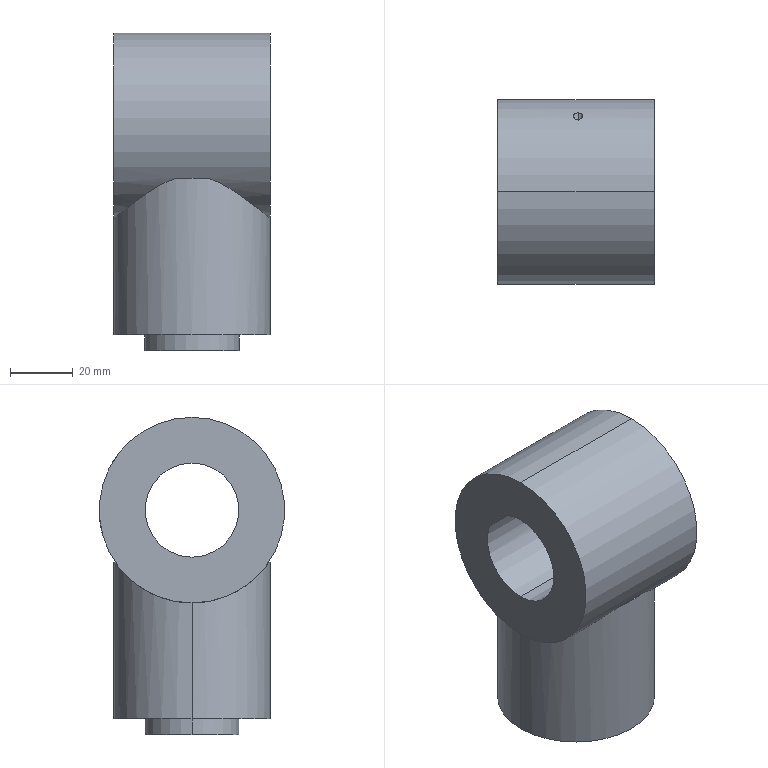Part | SolidWorks | features ICE 4, Extrusion 1, RefAxis 1 | 1 solid | 20 faces | box 50 x 59.155 x 101.162 mm | volume 183899 mm3 | cylinder 12 | plane 8 | commonest cylinder face diameters 3 x4 30 x4 50 x2 59.155 x2
STEP:
#1=CARTESIAN_POINT('',(-137.397,11.352,82.062));
#2=VERTEX_POINT('',#1);
#3=CARTESIAN_POINT('',(-137.397,9.243,85.062));
#4=VERTEX_POINT('',#3);
#5=CARTESIAN_POINT('',(-137.397,11.352,82.062));
#6=CARTESIAN_POINT('',(-137.508,11.352,82.062));
#7=CARTESIAN_POINT('',(-137.616,11.344,82.074));
#8=CARTESIAN_POINT('',(-137.827,11.315,82.121));
#9=CARTESIAN_POINT('',(-137.931,11.294,82.156));
#10=CARTESIAN_POINT('',(-138.122,11.239,82.245));
#11=CARTESIAN_POINT('',(-138.213,11.205,82.299));
#12=CARTESIAN_POINT('',(-138.377,11.127,82.422));
#13=CARTESIAN_POINT('',(-138.451,11.084,82.49));
#14=CARTESIAN_POINT('',(-138.649,10.942,82.712));
#15=CARTESIAN_POINT('',(-138.745,10.832,82.879));
#16=CARTESIAN_POINT('',(-138.871,10.598,83.228));
#17=CARTESIAN_POINT('',(-138.9,10.475,83.408));
#18=CARTESIAN_POINT('',(-138.894,10.223,83.767));
#19=CARTESIAN_POINT('',(-138.859,10.097,83.942));
#20=CARTESIAN_POINT('',(-138.727,9.849,84.279));
#21=CARTESIAN_POINT('',(-138.632,9.731,84.435));
#22=CARTESIAN_POINT('',(-138.374,9.516,84.716));
#23=CARTESIAN_POINT('',(-138.212,9.42,84.838));
#24=CARTESIAN_POINT('',(-137.928,9.317,84.969));
#25=CARTESIAN_POINT('',(-137.827,9.29,85.003));
#26=CARTESIAN_POINT('',(-137.615,9.252,85.05));
#27=CARTESIAN_POINT('',(-137.506,9.243,85.062));
#28=CARTESIAN_POINT('',(-137.397,9.243,85.062));
#29=B_SPLINE_CURVE_WITH_KNOTS('',3,(#5,#6,#7,#8,#9,#10,#11,#12,#13,#14,#15,#16,#17,#18,#19,#20,#21,#22,#23,#24,#25,#26,#27,#28),.UNSPECIFIED.,.F.,.F.,(4,2,2,2,2,2,2,2,2,2,2,4),(0.,0.0003267,0.0006535,0.0009802,0.001307,0.00196,0.002614,0.003267,0.003921,0.004574,0.004901,0.005228),.UNSPECIFIED.);
#30=EDGE_CURVE('',#2,#4,#29,.T.);
#31=ORIENTED_EDGE('',*,*,#30,.T.);
#32=CARTESIAN_POINT('',(-137.397,0.,85.062));
#33=VERTEX_POINT('',#32);
#34=CARTESIAN_POINT('',(-137.397,20.,85.062));
#35=DIRECTION('',(0.,-1.,0.));
#36=VECTOR('',#35,1000.);
#37=LINE('',#34,#36);
#38=EDGE_CURVE('',#4,#33,#37,.T.);
#39=ORIENTED_EDGE('',*,*,#38,.T.);
#40=CARTESIAN_POINT('',(-137.397,0.,82.062));
#41=VERTEX_POINT('',#40);
#42=CARTESIAN_POINT('',(-137.397,0.,83.562));
#43=DIRECTION('',(0.,1.,0.));
#44=DIRECTION('',(0.,0.,1.));
#45=AXIS2_PLACEMENT_3D('',#42,#43,#44);
#46=CIRCLE('',#45,1.5);
#47=EDGE_CURVE('',#41,#33,#46,.T.);
#48=ORIENTED_EDGE('',*,*,#47,.F.);
#49=CARTESIAN_POINT('',(-137.397,20.,82.062));
#50=DIRECTION('',(0.,-1.,0.));
#51=VECTOR('',#50,1000.);
#52=LINE('',#49,#51);
#53=EDGE_CURVE('',#2,#41,#52,.T.);
#54=ORIENTED_EDGE('',*,*,#53,.F.);
#55=EDGE_LOOP('',(#31,#39,#48,#54));
#56=FACE_OUTER_BOUND('',#55,.T.);
#57=CARTESIAN_POINT('',(-137.397,20.,83.562));
#58=DIRECTION('',(0.,-1.,0.));
#59=DIRECTION('',(0.,0.,-1.));
#60=AXIS2_PLACEMENT_3D('',#57,#58,#59);
#61=CYLINDRICAL_SURFACE('',#60,1.5);
#62=ADVANCED_FACE('',(#56),#61,.F.);
#63=CARTESIAN_POINT('',(-137.397,14.978,59.979));
#64=VERTEX_POINT('',#63);
#65=CARTESIAN_POINT('',(-137.397,15.504,62.979));
#66=VERTEX_POINT('',#65);
#67=CARTESIAN_POINT('',(-137.397,14.978,59.979));
#68=CARTESIAN_POINT('',(-137.497,14.978,59.979));
#69=CARTESIAN_POINT('',(-137.595,14.98,59.989));
#70=CARTESIAN_POINT('',(-137.788,14.989,60.027));
#71=CARTESIAN_POINT('',(-137.884,14.995,60.057));
#72=CARTESIAN_POINT('',(-138.066,15.012,60.133));
#73=CARTESIAN_POINT('',(-138.152,15.023,60.179));
#74=CARTESIAN_POINT('',(-138.315,15.047,60.289));
#75=CARTESIAN_POINT('',(-138.392,15.061,60.352));
#76=CARTESIAN_POINT('',(-138.598,15.105,60.56));
#77=CARTESIAN_POINT('',(-138.709,15.139,60.726));
#78=CARTESIAN_POINT('',(-138.857,15.209,61.084));
#79=CARTESIAN_POINT('',(-138.896,15.246,61.28));
#80=CARTESIAN_POINT('',(-138.897,15.297,61.571));
#81=CARTESIAN_POINT('',(-138.888,15.314,61.67));
#82=CARTESIAN_POINT('',(-138.851,15.345,61.861));
#83=CARTESIAN_POINT('',(-138.823,15.36,61.955));
#84=CARTESIAN_POINT('',(-138.749,15.388,62.136));
#85=CARTESIAN_POINT('',(-138.702,15.402,62.224));
#86=CARTESIAN_POINT('',(-138.595,15.425,62.387));
#87=CARTESIAN_POINT('',(-138.533,15.436,62.463));
#88=CARTESIAN_POINT('',(-138.323,15.465,62.675));
#89=CARTESIAN_POINT('',(-138.158,15.48,62.787));
#90=CARTESIAN_POINT('',(-137.884,15.494,62.901));
#91=CARTESIAN_POINT('',(-137.789,15.498,62.93));
#92=CARTESIAN_POINT('',(-137.596,15.503,62.969));
#93=CARTESIAN_POINT('',(-137.496,15.504,62.979));
#94=CARTESIAN_POINT('',(-137.397,15.504,62.979));
#95=B_SPLINE_CURVE_WITH_KNOTS('',3,(#67,#68,#69,#70,#71,#72,#73,#74,#75,#76,#77,#78,#79,#80,#81,#82,#83,#84,#85,#86,#87,#88,#89,#90,#91,#92,#93,#94),.UNSPECIFIED.,.F.,.F.,(4,2,2,2,2,2,2,2,2,2,2,2,2,4),(0.,0.0002954,0.0005909,0.0008863,0.001182,0.001773,0.002363,0.002659,0.002954,0.00325,0.003545,0.004136,0.004432,0.004727),.UNSPECIFIED.);
#96=EDGE_CURVE('',#64,#66,#95,.T.);
#97=ORIENTED_EDGE('',*,*,#96,.T.);
#98=CARTESIAN_POINT('',(-137.397,0.7071,62.979));
#99=VERTEX_POINT('',#98);
#100=CARTESIAN_POINT('',(-137.397,20.,62.979));
#101=DIRECTION('',(0.,-1.,0.));
#102=VECTOR('',#101,1000.);
#103=LINE('',#100,#102);
#104=EDGE_CURVE('',#66,#99,#103,.T.);
#105=ORIENTED_EDGE('',*,*,#104,.T.);
#106=CARTESIAN_POINT('',(-138.75,0.,60.832));
#107=VERTEX_POINT('',#106);
#108=CARTESIAN_POINT('',(-137.397,0.7071,62.979));
#109=CARTESIAN_POINT('',(-137.657,0.7071,62.979));
#110=CARTESIAN_POINT('',(-137.919,0.6901,62.909));
#111=CARTESIAN_POINT('',(-138.254,0.6397,62.716));
#112=CARTESIAN_POINT('',(-138.357,0.6187,62.638));
#113=CARTESIAN_POINT('',(-138.54,0.5685,62.458));
#114=CARTESIAN_POINT('',(-138.618,0.5398,62.359));
#115=CARTESIAN_POINT('',(-138.814,0.4414,62.033));
#116=CARTESIAN_POINT('',(-138.885,0.3613,61.787));
#117=CARTESIAN_POINT('',(-138.906,0.187,61.298));
#118=CARTESIAN_POINT('',(-138.856,0.09214,61.054));
#119=CARTESIAN_POINT('',(-138.75,0.,60.832));
#120=B_SPLINE_CURVE_WITH_KNOTS('',3,(#108,#109,#110,#111,#112,#113,#114,#115,#116,#117,#118,#119),.UNSPECIFIED.,.F.,.F.,(4,2,2,2,2,4),(0.003113,0.003889,0.004278,0.004666,0.005442,0.006219),.UNSPECIFIED.);
#121=EDGE_CURVE('',#99,#107,#120,.T.);
#122=ORIENTED_EDGE('',*,*,#121,.T.);
#123=CARTESIAN_POINT('',(-137.397,0.,59.979));
#124=VERTEX_POINT('',#123);
#125=CARTESIAN_POINT('',(-137.397,0.,61.479));
#126=DIRECTION('',(0.,1.,0.));
#127=DIRECTION('',(0.,0.,1.));
#128=AXIS2_PLACEMENT_3D('',#125,#126,#127);
#129=CIRCLE('',#128,1.5);
#130=EDGE_CURVE('',#124,#107,#129,.T.);
#131=ORIENTED_EDGE('',*,*,#130,.F.);
#132=CARTESIAN_POINT('',(-137.397,20.,59.979));
#133=DIRECTION('',(0.,-1.,0.));
#134=VECTOR('',#133,1000.);
#135=LINE('',#132,#134);
#136=EDGE_CURVE('',#64,#124,#135,.T.);
#137=ORIENTED_EDGE('',*,*,#136,.F.);
#138=EDGE_LOOP('',(#97,#105,#122,#131,#137));
#139=FACE_OUTER_BOUND('',#138,.T.);
#140=CARTESIAN_POINT('',(-137.397,20.,61.479));
#141=DIRECTION('',(0.,-1.,0.));
#142=DIRECTION('',(0.,0.,-1.));
#143=AXIS2_PLACEMENT_3D('',#140,#141,#142);
#144=CYLINDRICAL_SURFACE('',#143,1.5);
#145=ADVANCED_FACE('',(#139),#144,.F.);
#146=CARTESIAN_POINT('',(-153.045,-13.853,-5.));
#147=VERTEX_POINT('',#146);
#148=CARTESIAN_POINT('',(-123.045,-13.853,-5.));
#149=VERTEX_POINT('',#148);
#150=CARTESIAN_POINT('',(-138.045,-13.853,-5.));
#151=DIRECTION('',(0.,0.,-1.));
#152=DIRECTION('',(-1.,0.,0.));
#153=AXIS2_PLACEMENT_3D('',#150,#151,#152);
#154=CIRCLE('',#153,15.);
#155=EDGE_CURVE('',#147,#149,#154,.T.);
#156=ORIENTED_EDGE('',*,*,#155,.F.);
#157=CARTESIAN_POINT('',(-153.045,-13.853,0.));
#158=VERTEX_POINT('',#157);
#159=CARTESIAN_POINT('',(-153.045,-13.853,-5.));
#160=DIRECTION('',(0.,0.,1.));
#161=VECTOR('',#160,1000.);
#162=LINE('',#159,#161);
#163=EDGE_CURVE('',#147,#158,#162,.T.);
#164=ORIENTED_EDGE('',*,*,#163,.T.);
#165=CARTESIAN_POINT('',(-123.045,-13.853,0.));
#166=VERTEX_POINT('',#165);
#167=CARTESIAN_POINT('',(-138.045,-13.853,0.));
#168=DIRECTION('',(0.,0.,-1.));
#169=DIRECTION('',(1.,0.,0.));
#170=AXIS2_PLACEMENT_3D('',#167,#168,#169);
#171=CIRCLE('',#170,15.);
#172=EDGE_CURVE('',#158,#166,#171,.T.);
#173=ORIENTED_EDGE('',*,*,#172,.T.);
#174=CARTESIAN_POINT('',(-123.045,-13.853,-5.));
#175=DIRECTION('',(0.,0.,1.));
#176=VECTOR('',#175,1000.);
#177=LINE('',#174,#176);
#178=EDGE_CURVE('',#149,#166,#177,.T.);
#179=ORIENTED_EDGE('',*,*,#178,.F.);
#180=EDGE_LOOP('',(#156,#164,#173,#179));
#181=FACE_OUTER_BOUND('',#180,.T.);
#182=CARTESIAN_POINT('',(-138.045,-13.853,-5.));
#183=DIRECTION('',(0.,0.,1.));
#184=DIRECTION('',(1.,0.,0.));
#185=AXIS2_PLACEMENT_3D('',#182,#183,#184);
#186=CYLINDRICAL_SURFACE('',#185,15.);
#187=ADVANCED_FACE('',(#181),#186,.T.);
#188=CARTESIAN_POINT('',(-113.045,-13.853,37.007));
#189=VERTEX_POINT('',#188);
#190=CARTESIAN_POINT('',(-133.025,10.638,50.));
#191=VERTEX_POINT('',#190);
#192=CARTESIAN_POINT('',(-113.045,-13.853,37.007));
#193=CARTESIAN_POINT('',(-113.045,-13.087,37.007));
#194=CARTESIAN_POINT('',(-113.08,-12.321,37.036));
#195=CARTESIAN_POINT('',(-113.221,-10.79,37.156));
#196=CARTESIAN_POINT('',(-113.329,-10.02,37.246));
#197=CARTESIAN_POINT('',(-113.749,-7.767,37.6));
#198=CARTESIAN_POINT('',(-114.159,-6.326,37.944));
#199=CARTESIAN_POINT('',(-114.821,-4.591,38.492));
#200=CARTESIAN_POINT('',(-114.961,-4.247,38.608));
#201=CARTESIAN_POINT('',(-115.254,-3.57,38.849));
#202=CARTESIAN_POINT('',(-115.407,-3.238,38.975));
#203=CARTESIAN_POINT('',(-115.884,-2.258,39.365));
#204=CARTESIAN_POINT('',(-116.227,-1.627,39.643));
#205=CARTESIAN_POINT('',(-116.957,-0.4058,40.232));
#206=CARTESIAN_POINT('',(-117.346,0.1842,40.542));
#207=CARTESIAN_POINT('',(-118.167,1.325,41.19));
#208=CARTESIAN_POINT('',(-118.601,1.876,41.528));
#209=CARTESIAN_POINT('',(-119.945,3.447,42.561));
#210=CARTESIAN_POINT('',(-120.907,4.398,43.281));
#211=CARTESIAN_POINT('',(-122.448,5.697,44.382));
#212=CARTESIAN_POINT('',(-122.979,6.109,44.752));
#213=CARTESIAN_POINT('',(-124.076,6.892,45.494));
#214=CARTESIAN_POINT('',(-124.645,7.263,45.867));
#215=CARTESIAN_POINT('',(-126.399,8.311,46.972));
#216=CARTESIAN_POINT('',(-127.619,8.912,47.682));
#217=CARTESIAN_POINT('',(-129.554,9.671,48.65));
#218=CARTESIAN_POINT('',(-130.216,9.9,48.957));
#219=CARTESIAN_POINT('',(-131.585,10.308,49.52));
#220=CARTESIAN_POINT('',(-132.291,10.487,49.778));
#221=CARTESIAN_POINT('',(-133.025,10.638,50.));
#222=B_SPLINE_CURVE_WITH_KNOTS('',3,(#192,#193,#194,#195,#196,#197,#198,#199,#200,#201,#202,#203,#204,#205,#206,#207,#208,#209,#210,#211,#212,#213,#214,#215,#216,#217,#218,#219,#220,#221),.UNSPECIFIED.,.F.,.F.,(4,2,2,2,2,2,2,2,2,2,2,2,2,2,4),(0.03672,0.03901,0.0413,0.04589,0.04704,0.04819,0.05048,0.05278,0.05507,0.05966,0.06195,0.06425,0.06884,0.07113,0.07343),.UNSPECIFIED.);
#223=EDGE_CURVE('',#189,#191,#222,.T.);
#224=ORIENTED_EDGE('',*,*,#223,.F.);
#225=CARTESIAN_POINT('',(-113.045,-13.853,0.));
#226=VERTEX_POINT('',#225);
#227=CARTESIAN_POINT('',(-113.045,-13.853,50.));
#228=DIRECTION('',(0.,0.,-1.));
#229=VECTOR('',#228,1000.);
#230=LINE('',#227,#229);
#231=EDGE_CURVE('',#189,#226,#230,.T.);
#232=ORIENTED_EDGE('',*,*,#231,.T.);
#233=CARTESIAN_POINT('',(-163.045,-13.853,0.));
#234=VERTEX_POINT('',#233);
#235=CARTESIAN_POINT('',(-138.045,-13.853,0.));
#236=DIRECTION('',(0.,0.,1.));
#237=DIRECTION('',(1.,0.,0.));
#238=AXIS2_PLACEMENT_3D('',#235,#236,#237);
#239=CIRCLE('',#238,25.);
#240=EDGE_CURVE('',#226,#234,#239,.T.);
#241=ORIENTED_EDGE('',*,*,#240,.T.);
#242=CARTESIAN_POINT('',(-163.045,-13.853,37.007));
#243=VERTEX_POINT('',#242);
#244=CARTESIAN_POINT('',(-163.045,-13.853,50.));
#245=DIRECTION('',(0.,0.,-1.));
#246=VECTOR('',#245,1000.);
#247=LINE('',#244,#246);
#248=EDGE_CURVE('',#243,#234,#247,.T.);
#249=ORIENTED_EDGE('',*,*,#248,.F.);
#250=CARTESIAN_POINT('',(-143.064,10.638,50.));
#251=VERTEX_POINT('',#250);
#252=CARTESIAN_POINT('',(-143.064,10.638,50.));
#253=CARTESIAN_POINT('',(-143.798,10.487,49.778));
#254=CARTESIAN_POINT('',(-144.504,10.309,49.521));
#255=CARTESIAN_POINT('',(-145.872,9.9,48.957));
#256=CARTESIAN_POINT('',(-146.535,9.671,48.651));
#257=CARTESIAN_POINT('',(-147.826,9.164,48.005));
#258=CARTESIAN_POINT('',(-148.454,8.887,47.665));
#259=CARTESIAN_POINT('',(-149.682,8.284,46.963));
#260=CARTESIAN_POINT('',(-150.282,7.958,46.6));
#261=CARTESIAN_POINT('',(-152.037,6.909,45.494));
#262=CARTESIAN_POINT('',(-153.131,6.127,44.746));
#263=CARTESIAN_POINT('',(-154.677,4.823,43.642));
#264=CARTESIAN_POINT('',(-155.177,4.367,43.277));
#265=CARTESIAN_POINT('',(-156.144,3.406,42.557));
#266=CARTESIAN_POINT('',(-156.613,2.901,42.201));
#267=CARTESIAN_POINT('',(-157.961,1.321,41.164));
#268=CARTESIAN_POINT('',(-158.776,0.1904,40.518));
#269=CARTESIAN_POINT('',(-159.867,-1.635,39.64));
#270=CARTESIAN_POINT('',(-160.209,-2.265,39.362));
#271=CARTESIAN_POINT('',(-160.845,-3.573,38.842));
#272=CARTESIAN_POINT('',(-161.14,-4.253,38.598));
#273=CARTESIAN_POINT('',(-161.931,-6.329,37.943));
#274=CARTESIAN_POINT('',(-162.341,-7.768,37.6));
#275=CARTESIAN_POINT('',(-162.761,-10.019,37.246));
#276=CARTESIAN_POINT('',(-162.868,-10.789,37.156));
#277=CARTESIAN_POINT('',(-163.01,-12.321,37.036));
#278=CARTESIAN_POINT('',(-163.045,-13.087,37.007));
#279=CARTESIAN_POINT('',(-163.045,-13.853,37.007));
#280=B_SPLINE_CURVE_WITH_KNOTS('',3,(#252,#253,#254,#255,#256,#257,#258,#259,#260,#261,#262,#263,#264,#265,#266,#267,#268,#269,#270,#271,#272,#273,#274,#275,#276,#277,#278,#279),.UNSPECIFIED.,.F.,.F.,(4,2,2,2,2,2,2,2,2,2,2,2,2,4),(0.,0.002295,0.00459,0.006884,0.009179,0.01377,0.01606,0.01836,0.02295,0.02524,0.02754,0.03213,0.03442,0.03672),.UNSPECIFIED.);
#281=EDGE_CURVE('',#251,#243,#280,.T.);
#282=ORIENTED_EDGE('',*,*,#281,.F.);
#283=CARTESIAN_POINT('',(-138.045,-13.853,50.));
#284=DIRECTION('',(0.,0.,1.));
#285=DIRECTION('',(1.,0.,0.));
#286=AXIS2_PLACEMENT_3D('',#283,#284,#285);
#287=CIRCLE('',#286,25.);
#288=EDGE_CURVE('',#191,#251,#287,.T.);
#289=ORIENTED_EDGE('',*,*,#288,.F.);
#290=EDGE_LOOP('',(#224,#232,#241,#249,#282,#289));
#291=FACE_OUTER_BOUND('',#290,.T.);
#292=CARTESIAN_POINT('',(-138.045,-13.853,50.));
#293=DIRECTION('',(0.,0.,-1.));
#294=DIRECTION('',(-1.,0.,0.));
#295=AXIS2_PLACEMENT_3D('',#292,#293,#294);
#296=CYLINDRICAL_SURFACE('',#295,25.);
#297=ADVANCED_FACE('',(#291),#296,.T.);
#298=CARTESIAN_POINT('',(-113.045,-13.853,51.584));
#299=VERTEX_POINT('',#298);
#300=CARTESIAN_POINT('',(-113.045,-13.853,81.584));
#301=VERTEX_POINT('',#300);
#302=CARTESIAN_POINT('',(-113.045,-13.853,66.584));
#303=DIRECTION('',(-1.,0.,0.));
#304=DIRECTION('',(0.,0.,-1.));
#305=AXIS2_PLACEMENT_3D('',#302,#303,#304);
#306=CIRCLE('',#305,15.);
#307=EDGE_CURVE('',#299,#301,#306,.T.);
#308=ORIENTED_EDGE('',*,*,#307,.F.);
#309=CARTESIAN_POINT('',(-163.045,-13.853,51.584));
#310=VERTEX_POINT('',#309);
#311=CARTESIAN_POINT('',(-113.044,-13.853,51.584));
#312=DIRECTION('',(-1.,0.,0.));
#313=VECTOR('',#312,1000.);
#314=LINE('',#311,#313);
#315=EDGE_CURVE('',#299,#310,#314,.T.);
#316=ORIENTED_EDGE('',*,*,#315,.T.);
#317=CARTESIAN_POINT('',(-163.045,-13.853,81.584));
#318=VERTEX_POINT('',#317);
#319=CARTESIAN_POINT('',(-163.045,-13.853,66.584));
#320=DIRECTION('',(-1.,0.,0.));
#321=DIRECTION('',(0.,0.,1.));
#322=AXIS2_PLACEMENT_3D('',#319,#320,#321);
#323=CIRCLE('',#322,15.);
#324=EDGE_CURVE('',#310,#318,#323,.T.);
#325=ORIENTED_EDGE('',*,*,#324,.T.);
#326=CARTESIAN_POINT('',(-113.044,-13.853,81.584));
#327=DIRECTION('',(-1.,0.,0.));
#328=VECTOR('',#327,1000.);
#329=LINE('',#326,#328);
#330=EDGE_CURVE('',#301,#318,#329,.T.);
#331=ORIENTED_EDGE('',*,*,#330,.F.);
#332=EDGE_LOOP('',(#308,#316,#325,#331));
#333=FACE_OUTER_BOUND('',#332,.T.);
#334=CARTESIAN_POINT('',(-113.044,-13.853,66.584));
#335=DIRECTION('',(-1.,0.,0.));
#336=DIRECTION('',(0.,0.,1.));
#337=AXIS2_PLACEMENT_3D('',#334,#335,#336);
#338=CYLINDRICAL_SURFACE('',#337,15.);
#339=ADVANCED_FACE('',(#333),#338,.F.);
#340=CARTESIAN_POINT('',(-113.045,-13.853,96.162));
#341=VERTEX_POINT('',#340);
#342=CARTESIAN_POINT('',(-113.045,-13.853,66.584));
#343=DIRECTION('',(1.,0.,0.));
#344=DIRECTION('',(0.,0.,-1.));
#345=AXIS2_PLACEMENT_3D('',#342,#343,#344);
#346=CIRCLE('',#345,29.578);
#347=EDGE_CURVE('',#341,#189,#346,.T.);
#348=ORIENTED_EDGE('',*,*,#347,.F.);
#349=CARTESIAN_POINT('',(-163.045,-13.853,96.162));
#350=VERTEX_POINT('',#349);
#351=CARTESIAN_POINT('',(-113.045,-13.853,96.162));
#352=DIRECTION('',(-1.,0.,0.));
#353=VECTOR('',#352,1000.);
#354=LINE('',#351,#353);
#355=EDGE_CURVE('',#341,#350,#354,.T.);
#356=ORIENTED_EDGE('',*,*,#355,.T.);
#357=CARTESIAN_POINT('',(-163.045,-13.853,66.584));
#358=DIRECTION('',(1.,0.,0.));
#359=DIRECTION('',(0.,0.,-1.));
#360=AXIS2_PLACEMENT_3D('',#357,#358,#359);
#361=CIRCLE('',#360,29.578);
#362=EDGE_CURVE('',#350,#243,#361,.T.);
#363=ORIENTED_EDGE('',*,*,#362,.T.);
#364=CARTESIAN_POINT('',(-143.064,-38.344,50.));
#365=VERTEX_POINT('',#364);
#366=CARTESIAN_POINT('',(-163.045,-13.853,37.007));
#367=CARTESIAN_POINT('',(-163.045,-14.619,37.007));
#368=CARTESIAN_POINT('',(-163.01,-15.385,37.036));
#369=CARTESIAN_POINT('',(-162.868,-16.917,37.156));
#370=CARTESIAN_POINT('',(-162.761,-17.687,37.246));
#371=CARTESIAN_POINT('',(-162.341,-19.939,37.6));
#372=CARTESIAN_POINT('',(-161.931,-21.381,37.944));
#373=CARTESIAN_POINT('',(-161.269,-23.115,38.492));
#374=CARTESIAN_POINT('',(-161.128,-23.46,38.608));
#375=CARTESIAN_POINT('',(-160.835,-24.136,38.849));
#376=CARTESIAN_POINT('',(-160.682,-24.468,38.975));
#377=CARTESIAN_POINT('',(-160.205,-25.448,39.365));
#378=CARTESIAN_POINT('',(-159.863,-26.079,39.643));
#379=CARTESIAN_POINT('',(-159.132,-27.301,40.232));
#380=CARTESIAN_POINT('',(-158.744,-27.89,40.542));
#381=CARTESIAN_POINT('',(-157.922,-29.032,41.19));
#382=CARTESIAN_POINT('',(-157.489,-29.582,41.528));
#383=CARTESIAN_POINT('',(-156.144,-31.153,42.561));
#384=CARTESIAN_POINT('',(-155.183,-32.104,43.281));
#385=CARTESIAN_POINT('',(-153.641,-33.403,44.382));
#386=CARTESIAN_POINT('',(-153.11,-33.815,44.752));
#387=CARTESIAN_POINT('',(-152.013,-34.598,45.494));
#388=CARTESIAN_POINT('',(-151.445,-34.97,45.867));
#389=CARTESIAN_POINT('',(-149.69,-36.017,46.972));
#390=CARTESIAN_POINT('',(-148.47,-36.618,47.682));
#391=CARTESIAN_POINT('',(-146.536,-37.377,48.65));
#392=CARTESIAN_POINT('',(-145.873,-37.607,48.957));
#393=CARTESIAN_POINT('',(-144.505,-38.015,49.52));
#394=CARTESIAN_POINT('',(-143.799,-38.193,49.778));
#395=CARTESIAN_POINT('',(-143.064,-38.344,50.));
#396=B_SPLINE_CURVE_WITH_KNOTS('',3,(#366,#367,#368,#369,#370,#371,#372,#373,#374,#375,#376,#377,#378,#379,#380,#381,#382,#383,#384,#385,#386,#387,#388,#389,#390,#391,#392,#393,#394,#395),.UNSPECIFIED.,.F.,.F.,(4,2,2,2,2,2,2,2,2,2,2,2,2,2,4),(0.03672,0.03901,0.0413,0.04589,0.04704,0.04819,0.05048,0.05278,0.05507,0.05966,0.06195,0.06425,0.06884,0.07113,0.07343),.UNSPECIFIED.);
#397=EDGE_CURVE('',#243,#365,#396,.T.);
#398=ORIENTED_EDGE('',*,*,#397,.T.);
#399=CARTESIAN_POINT('',(-133.025,-38.344,50.));
#400=VERTEX_POINT('',#399);
#401=CARTESIAN_POINT('',(-113.045,-38.344,50.));
#402=DIRECTION('',(-1.,0.,0.));
#403=VECTOR('',#402,1000.);
#404=LINE('',#401,#403);
#405=EDGE_CURVE('',#400,#365,#404,.T.);
#406=ORIENTED_EDGE('',*,*,#405,.F.);
#407=CARTESIAN_POINT('',(-133.025,-38.344,50.));
#408=CARTESIAN_POINT('',(-132.291,-38.194,49.778));
#409=CARTESIAN_POINT('',(-131.585,-38.015,49.521));
#410=CARTESIAN_POINT('',(-130.217,-37.607,48.957));
#411=CARTESIAN_POINT('',(-129.554,-37.377,48.651));
#412=CARTESIAN_POINT('',(-128.263,-36.871,48.005));
#413=CARTESIAN_POINT('',(-127.635,-36.593,47.665));
#414=CARTESIAN_POINT('',(-126.408,-35.99,46.963));
#415=CARTESIAN_POINT('',(-125.808,-35.664,46.6));
#416=CARTESIAN_POINT('',(-124.053,-34.616,45.494));
#417=CARTESIAN_POINT('',(-122.958,-33.834,44.746));
#418=CARTESIAN_POINT('',(-121.412,-32.53,43.642));
#419=CARTESIAN_POINT('',(-120.913,-32.073,43.277));
#420=CARTESIAN_POINT('',(-119.946,-31.113,42.557));
#421=CARTESIAN_POINT('',(-119.476,-30.607,42.201));
#422=CARTESIAN_POINT('',(-118.128,-29.027,41.164));
#423=CARTESIAN_POINT('',(-117.313,-27.897,40.518));
#424=CARTESIAN_POINT('',(-116.222,-26.072,39.64));
#425=CARTESIAN_POINT('',(-115.881,-25.442,39.362));
#426=CARTESIAN_POINT('',(-115.245,-24.134,38.842));
#427=CARTESIAN_POINT('',(-114.949,-23.453,38.598));
#428=CARTESIAN_POINT('',(-114.158,-21.378,37.943));
#429=CARTESIAN_POINT('',(-113.749,-19.939,37.6));
#430=CARTESIAN_POINT('',(-113.329,-17.687,37.246));
#431=CARTESIAN_POINT('',(-113.221,-16.917,37.156));
#432=CARTESIAN_POINT('',(-113.08,-15.385,37.036));
#433=CARTESIAN_POINT('',(-113.045,-14.619,37.007));
#434=CARTESIAN_POINT('',(-113.045,-13.853,37.007));
#435=B_SPLINE_CURVE_WITH_KNOTS('',3,(#407,#408,#409,#410,#411,#412,#413,#414,#415,#416,#417,#418,#419,#420,#421,#422,#423,#424,#425,#426,#427,#428,#429,#430,#431,#432,#433,#434),.UNSPECIFIED.,.F.,.F.,(4,2,2,2,2,2,2,2,2,2,2,2,2,4),(0.,0.002295,0.00459,0.006884,0.009179,0.01377,0.01606,0.01836,0.02295,0.02524,0.02754,0.03213,0.03442,0.03672),.UNSPECIFIED.);
#436=EDGE_CURVE('',#400,#189,#435,.T.);
#437=ORIENTED_EDGE('',*,*,#436,.T.);
#438=EDGE_LOOP('',(#348,#356,#363,#398,#406,#437));
#439=FACE_OUTER_BOUND('',#438,.T.);
#440=CARTESIAN_POINT('',(-113.045,-13.853,66.584));
#441=DIRECTION('',(-1.,0.,0.));
#442=DIRECTION('',(0.,0.,1.));
#443=AXIS2_PLACEMENT_3D('',#440,#441,#442);
#444=CYLINDRICAL_SURFACE('',#443,29.578);
#445=ADVANCED_FACE('',(#439),#444,.T.);
#446=ORIENTED_EDGE('',*,*,#355,.F.);
#447=CARTESIAN_POINT('',(-113.045,-13.853,66.584));
#448=DIRECTION('',(1.,0.,0.));
#449=DIRECTION('',(0.,0.,-1.));
#450=AXIS2_PLACEMENT_3D('',#447,#448,#449);
#451=CIRCLE('',#450,29.578);
#452=EDGE_CURVE('',#189,#341,#451,.T.);
#453=ORIENTED_EDGE('',*,*,#452,.F.);
#454=ORIENTED_EDGE('',*,*,#223,.T.);
#455=CARTESIAN_POINT('',(-113.045,10.638,50.));
#456=DIRECTION('',(1.,0.,0.));
#457=VECTOR('',#456,1000.);
#458=LINE('',#455,#457);
#459=EDGE_CURVE('',#251,#191,#458,.T.);
#460=ORIENTED_EDGE('',*,*,#459,.F.);
#461=ORIENTED_EDGE('',*,*,#281,.T.);
#462=CARTESIAN_POINT('',(-163.045,-13.853,66.584));
#463=DIRECTION('',(1.,0.,0.));
#464=DIRECTION('',(0.,0.,-1.));
#465=AXIS2_PLACEMENT_3D('',#462,#463,#464);
#466=CIRCLE('',#465,29.578);
#467=EDGE_CURVE('',#243,#350,#466,.T.);
#468=ORIENTED_EDGE('',*,*,#467,.T.);
#469=EDGE_LOOP('',(#446,#453,#454,#460,#461,#468));
#470=FACE_OUTER_BOUND('',#469,.T.);
#471=ORIENTED_EDGE('',*,*,#30,.F.);
#472=CARTESIAN_POINT('',(-137.397,9.243,85.062));
#473=CARTESIAN_POINT('',(-137.288,9.243,85.062));
#474=CARTESIAN_POINT('',(-137.177,9.253,85.05));
#475=CARTESIAN_POINT('',(-136.967,9.29,85.003));
#476=CARTESIAN_POINT('',(-136.865,9.317,84.968));
#477=CARTESIAN_POINT('',(-136.582,9.42,84.838));
#478=CARTESIAN_POINT('',(-136.42,9.516,84.716));
#479=CARTESIAN_POINT('',(-136.162,9.731,84.435));
#480=CARTESIAN_POINT('',(-136.065,9.851,84.276));
#481=CARTESIAN_POINT('',(-135.934,10.099,83.938));
#482=CARTESIAN_POINT('',(-135.9,10.226,83.763));
#483=CARTESIAN_POINT('',(-135.895,10.477,83.404));
#484=CARTESIAN_POINT('',(-135.924,10.601,83.225));
#485=CARTESIAN_POINT('',(-136.018,10.775,82.965));
#486=CARTESIAN_POINT('',(-136.058,10.832,82.879));
#487=CARTESIAN_POINT('',(-136.155,10.939,82.715));
#488=CARTESIAN_POINT('',(-136.212,10.99,82.637));
#489=CARTESIAN_POINT('',(-136.343,11.084,82.49));
#490=CARTESIAN_POINT('',(-136.419,11.128,82.42));
#491=CARTESIAN_POINT('',(-136.582,11.205,82.299));
#492=CARTESIAN_POINT('',(-136.67,11.238,82.245));
#493=CARTESIAN_POINT('',(-136.959,11.321,82.112));
#494=CARTESIAN_POINT('',(-137.176,11.352,82.062));
#495=CARTESIAN_POINT('',(-137.397,11.352,82.062));
#496=B_SPLINE_CURVE_WITH_KNOTS('',3,(#472,#473,#474,#475,#476,#477,#478,#479,#480,#481,#482,#483,#484,#485,#486,#487,#488,#489,#490,#491,#492,#493,#494,#495),.UNSPECIFIED.,.F.,.F.,(4,2,2,2,2,2,2,2,2,2,2,4),(0.005228,0.005554,0.00588,0.006532,0.007185,0.007837,0.008489,0.008815,0.009142,0.009468,0.009794,0.01045),.UNSPECIFIED.);
#497=EDGE_CURVE('',#4,#2,#496,.T.);
#498=ORIENTED_EDGE('',*,*,#497,.F.);
#499=EDGE_LOOP('',(#471,#498));
#500=FACE_BOUND('',#499,.T.);
#501=ORIENTED_EDGE('',*,*,#96,.F.);
#502=CARTESIAN_POINT('',(-137.397,15.504,62.979));
#503=CARTESIAN_POINT('',(-137.2,15.504,62.979));
#504=CARTESIAN_POINT('',(-137.001,15.499,62.939));
#505=CARTESIAN_POINT('',(-136.638,15.48,62.787));
#506=CARTESIAN_POINT('',(-136.47,15.465,62.674));
#507=CARTESIAN_POINT('',(-136.263,15.436,62.465));
#508=CARTESIAN_POINT('',(-136.2,15.425,62.388));
#509=CARTESIAN_POINT('',(-136.091,15.402,62.224));
#510=CARTESIAN_POINT('',(-136.046,15.389,62.138));
#511=CARTESIAN_POINT('',(-135.934,15.346,61.865));
#512=CARTESIAN_POINT('',(-135.896,15.314,61.671));
#513=CARTESIAN_POINT('',(-135.897,15.263,61.377));
#514=CARTESIAN_POINT('',(-135.907,15.245,61.28));
#515=CARTESIAN_POINT('',(-135.945,15.21,61.09));
#516=CARTESIAN_POINT('',(-135.974,15.192,60.996));
#517=CARTESIAN_POINT('',(-136.048,15.157,60.815));
#518=CARTESIAN_POINT('',(-136.094,15.14,60.73));
#519=CARTESIAN_POINT('',(-136.201,15.106,60.568));
#520=CARTESIAN_POINT('',(-136.264,15.09,60.491));
#521=CARTESIAN_POINT('',(-136.47,15.046,60.283));
#522=CARTESIAN_POINT('',(-136.637,15.021,60.171));
#523=CARTESIAN_POINT('',(-136.999,14.987,60.019));
#524=CARTESIAN_POINT('',(-137.197,14.978,59.979));
#525=CARTESIAN_POINT('',(-137.397,14.978,59.979));
#526=B_SPLINE_CURVE_WITH_KNOTS('',3,(#502,#503,#504,#505,#506,#507,#508,#509,#510,#511,#512,#513,#514,#515,#516,#517,#518,#519,#520,#521,#522,#523,#524,#525),.UNSPECIFIED.,.F.,.F.,(4,2,2,2,2,2,2,2,2,2,2,4),(0.004727,0.005318,0.005908,0.006204,0.006499,0.00709,0.007385,0.007681,0.007976,0.008271,0.008862,0.009453),.UNSPECIFIED.);
#527=EDGE_CURVE('',#66,#64,#526,.T.);
#528=ORIENTED_EDGE('',*,*,#527,.F.);
#529=EDGE_LOOP('',(#501,#528));
#530=FACE_BOUND('',#529,.T.);
#531=CARTESIAN_POINT('',(-113.045,-13.853,66.584));
#532=DIRECTION('',(-1.,0.,0.));
#533=DIRECTION('',(0.,0.,1.));
#534=AXIS2_PLACEMENT_3D('',#531,#532,#533);
#535=CYLINDRICAL_SURFACE('',#534,29.578);
#536=ADVANCED_FACE('',(#470,#500,#530),#535,.T.);
#537=ORIENTED_EDGE('',*,*,#315,.F.);
#538=CARTESIAN_POINT('',(-113.045,-13.853,66.584));
#539=DIRECTION('',(-1.,0.,0.));
#540=DIRECTION('',(0.,0.,-1.));
#541=AXIS2_PLACEMENT_3D('',#538,#539,#540);
#542=CIRCLE('',#541,15.);
#543=EDGE_CURVE('',#301,#299,#542,.T.);
#544=ORIENTED_EDGE('',*,*,#543,.F.);
#545=ORIENTED_EDGE('',*,*,#330,.T.);
#546=CARTESIAN_POINT('',(-163.045,-13.853,66.584));
#547=DIRECTION('',(-1.,0.,0.));
#548=DIRECTION('',(0.,0.,1.));
#549=AXIS2_PLACEMENT_3D('',#546,#547,#548);
#550=CIRCLE('',#549,15.);
#551=EDGE_CURVE('',#318,#310,#550,.T.);
#552=ORIENTED_EDGE('',*,*,#551,.T.);
#553=EDGE_LOOP('',(#537,#544,#545,#552));
#554=FACE_OUTER_BOUND('',#553,.T.);
#555=CARTESIAN_POINT('',(-136.044,0.,60.832));
#556=VERTEX_POINT('',#555);
#557=CARTESIAN_POINT('',(-136.044,0.,60.832));
#558=CARTESIAN_POINT('',(-135.99,0.04615,60.943));
#559=CARTESIAN_POINT('',(-135.952,0.09238,61.058));
#560=CARTESIAN_POINT('',(-135.903,0.1844,61.296));
#561=CARTESIAN_POINT('',(-135.893,0.2305,61.42));
#562=CARTESIAN_POINT('',(-135.909,0.3613,61.787));
#563=CARTESIAN_POINT('',(-135.98,0.4414,62.033));
#564=CARTESIAN_POINT('',(-136.174,0.5392,62.357));
#565=CARTESIAN_POINT('',(-136.254,0.5687,62.459));
#566=CARTESIAN_POINT('',(-136.436,0.6185,62.637));
#567=CARTESIAN_POINT('',(-136.54,0.6397,62.716));
#568=CARTESIAN_POINT('',(-136.877,0.6903,62.909));
#569=CARTESIAN_POINT('',(-137.136,0.7071,62.979));
#570=CARTESIAN_POINT('',(-137.397,0.7071,62.979));
#571=B_SPLINE_CURVE_WITH_KNOTS('',3,(#557,#558,#559,#560,#561,#562,#563,#564,#565,#566,#567,#568,#569,#570),.UNSPECIFIED.,.F.,.F.,(4,2,2,2,2,2,4),(0.,0.0003891,0.0007781,0.001556,0.001945,0.002334,0.003113),.UNSPECIFIED.);
#572=EDGE_CURVE('',#556,#99,#571,.T.);
#573=ORIENTED_EDGE('',*,*,#572,.F.);
#574=CARTESIAN_POINT('',(-113.044,0.,60.832));
#575=DIRECTION('',(1.,0.,0.));
#576=VECTOR('',#575,1000.);
#577=LINE('',#574,#576);
#578=EDGE_CURVE('',#107,#556,#577,.T.);
#579=ORIENTED_EDGE('',*,*,#578,.F.);
#580=ORIENTED_EDGE('',*,*,#121,.F.);
#581=EDGE_LOOP('',(#573,#579,#580));
#582=FACE_BOUND('',#581,.T.);
#583=CARTESIAN_POINT('',(-113.044,-13.853,66.584));
#584=DIRECTION('',(-1.,0.,0.));
#585=DIRECTION('',(0.,0.,1.));
#586=AXIS2_PLACEMENT_3D('',#583,#584,#585);
#587=CYLINDRICAL_SURFACE('',#586,15.);
#588=ADVANCED_FACE('',(#554,#582),#587,.F.);
#589=ORIENTED_EDGE('',*,*,#231,.F.);
#590=ORIENTED_EDGE('',*,*,#436,.F.);
#591=CARTESIAN_POINT('',(-138.045,-13.853,50.));
#592=DIRECTION('',(0.,0.,1.));
#593=DIRECTION('',(1.,0.,0.));
#594=AXIS2_PLACEMENT_3D('',#591,#592,#593);
#595=CIRCLE('',#594,25.);
#596=EDGE_CURVE('',#365,#400,#595,.T.);
#597=ORIENTED_EDGE('',*,*,#596,.F.);
#598=ORIENTED_EDGE('',*,*,#397,.F.);
#599=ORIENTED_EDGE('',*,*,#248,.T.);
#600=CARTESIAN_POINT('',(-138.045,-13.853,0.));
#601=DIRECTION('',(0.,0.,1.));
#602=DIRECTION('',(1.,0.,0.));
#603=AXIS2_PLACEMENT_3D('',#600,#601,#602);
#604=CIRCLE('',#603,25.);
#605=EDGE_CURVE('',#234,#226,#604,.T.);
#606=ORIENTED_EDGE('',*,*,#605,.T.);
#607=EDGE_LOOP('',(#589,#590,#597,#598,#599,#606));
#608=FACE_OUTER_BOUND('',#607,.T.);
#609=CARTESIAN_POINT('',(-138.045,-13.853,50.));
#610=DIRECTION('',(0.,0.,-1.));
#611=DIRECTION('',(-1.,0.,0.));
#612=AXIS2_PLACEMENT_3D('',#609,#610,#611);
#613=CYLINDRICAL_SURFACE('',#612,25.);
#614=ADVANCED_FACE('',(#608),#613,.T.);
#615=ORIENTED_EDGE('',*,*,#288,.T.);
#616=ORIENTED_EDGE('',*,*,#459,.T.);
#617=EDGE_LOOP('',(#615,#616));
#618=FACE_OUTER_BOUND('',#617,.T.);
#619=CARTESIAN_POINT('',(-138.045,-13.853,50.));
#620=DIRECTION('',(0.,0.,1.));
#621=DIRECTION('',(1.,0.,0.));
#622=AXIS2_PLACEMENT_3D('',#619,#620,#621);
#623=PLANE('',#622);
#624=ADVANCED_FACE('',(#618),#623,.T.);
#625=ORIENTED_EDGE('',*,*,#596,.T.);
#626=ORIENTED_EDGE('',*,*,#405,.T.);
#627=EDGE_LOOP('',(#625,#626));
#628=FACE_OUTER_BOUND('',#627,.T.);
#629=CARTESIAN_POINT('',(-138.045,-13.853,50.));
#630=DIRECTION('',(0.,0.,1.));
#631=DIRECTION('',(1.,0.,0.));
#632=AXIS2_PLACEMENT_3D('',#629,#630,#631);
#633=PLANE('',#632);
#634=ADVANCED_FACE('',(#628),#633,.T.);
#635=CARTESIAN_POINT('',(-138.045,-13.853,0.));
#636=DIRECTION('',(0.,0.,-1.));
#637=DIRECTION('',(1.,0.,0.));
#638=AXIS2_PLACEMENT_3D('',#635,#636,#637);
#639=CIRCLE('',#638,15.);
#640=EDGE_CURVE('',#166,#158,#639,.T.);
#641=ORIENTED_EDGE('',*,*,#640,.F.);
#642=ORIENTED_EDGE('',*,*,#172,.F.);
#643=EDGE_LOOP('',(#641,#642));
#644=FACE_BOUND('',#643,.T.);
#645=ORIENTED_EDGE('',*,*,#605,.F.);
#646=ORIENTED_EDGE('',*,*,#240,.F.);
#647=EDGE_LOOP('',(#645,#646));
#648=FACE_OUTER_BOUND('',#647,.T.);
#649=CARTESIAN_POINT('',(-138.045,-13.853,0.));
#650=DIRECTION('',(0.,0.,1.));
#651=DIRECTION('',(1.,0.,0.));
#652=AXIS2_PLACEMENT_3D('',#649,#650,#651);
#653=PLANE('',#652);
#654=ADVANCED_FACE('',(#644,#648),#653,.F.);
#655=ORIENTED_EDGE('',*,*,#543,.T.);
#656=ORIENTED_EDGE('',*,*,#307,.T.);
#657=EDGE_LOOP('',(#655,#656));
#658=FACE_BOUND('',#657,.T.);
#659=ORIENTED_EDGE('',*,*,#452,.T.);
#660=ORIENTED_EDGE('',*,*,#347,.T.);
#661=EDGE_LOOP('',(#659,#660));
#662=FACE_OUTER_BOUND('',#661,.T.);
#663=CARTESIAN_POINT('',(-113.045,-13.853,66.584));
#664=DIRECTION('',(1.,0.,0.));
#665=DIRECTION('',(0.,0.,-1.));
#666=AXIS2_PLACEMENT_3D('',#663,#664,#665);
#667=PLANE('',#666);
#668=ADVANCED_FACE('',(#658,#662),#667,.T.);
#669=ORIENTED_EDGE('',*,*,#551,.F.);
#670=ORIENTED_EDGE('',*,*,#324,.F.);
#671=EDGE_LOOP('',(#669,#670));
#672=FACE_BOUND('',#671,.T.);
#673=ORIENTED_EDGE('',*,*,#467,.F.);
#674=ORIENTED_EDGE('',*,*,#362,.F.);
#675=EDGE_LOOP('',(#673,#674));
#676=FACE_OUTER_BOUND('',#675,.T.);
#677=CARTESIAN_POINT('',(-163.045,-13.853,66.584));
#678=DIRECTION('',(1.,0.,0.));
#679=DIRECTION('',(0.,0.,-1.));
#680=AXIS2_PLACEMENT_3D('',#677,#678,#679);
#681=PLANE('',#680);
#682=ADVANCED_FACE('',(#672,#676),#681,.F.);
#683=ORIENTED_EDGE('',*,*,#163,.F.);
#684=CARTESIAN_POINT('',(-138.045,-13.853,-5.));
#685=DIRECTION('',(0.,0.,-1.));
#686=DIRECTION('',(-1.,0.,0.));
#687=AXIS2_PLACEMENT_3D('',#684,#685,#686);
#688=CIRCLE('',#687,15.);
#689=EDGE_CURVE('',#149,#147,#688,.T.);
#690=ORIENTED_EDGE('',*,*,#689,.F.);
#691=ORIENTED_EDGE('',*,*,#178,.T.);
#692=ORIENTED_EDGE('',*,*,#640,.T.);
#693=EDGE_LOOP('',(#683,#690,#691,#692));
#694=FACE_OUTER_BOUND('',#693,.T.);
#695=CARTESIAN_POINT('',(-138.045,-13.853,-5.));
#696=DIRECTION('',(0.,0.,1.));
#697=DIRECTION('',(1.,0.,0.));
#698=AXIS2_PLACEMENT_3D('',#695,#696,#697);
#699=CYLINDRICAL_SURFACE('',#698,15.);
#700=ADVANCED_FACE('',(#694),#699,.T.);
#701=ORIENTED_EDGE('',*,*,#689,.T.);
#702=ORIENTED_EDGE('',*,*,#155,.T.);
#703=EDGE_LOOP('',(#701,#702));
#704=FACE_OUTER_BOUND('',#703,.T.);
#705=CARTESIAN_POINT('',(-138.045,-13.853,-5.));
#706=DIRECTION('',(0.,0.,-1.));
#707=DIRECTION('',(-1.,0.,0.));
#708=AXIS2_PLACEMENT_3D('',#705,#706,#707);
#709=PLANE('',#708);
#710=ADVANCED_FACE('',(#704),#709,.T.);
#711=ORIENTED_EDGE('',*,*,#104,.F.);
#712=ORIENTED_EDGE('',*,*,#527,.T.);
#713=ORIENTED_EDGE('',*,*,#136,.T.);
#714=CARTESIAN_POINT('',(-137.397,0.,61.479));
#715=DIRECTION('',(0.,1.,0.));
#716=DIRECTION('',(0.,0.,1.));
#717=AXIS2_PLACEMENT_3D('',#714,#715,#716);
#718=CIRCLE('',#717,1.5);
#719=EDGE_CURVE('',#556,#124,#718,.T.);
#720=ORIENTED_EDGE('',*,*,#719,.F.);
#721=ORIENTED_EDGE('',*,*,#572,.T.);
#722=EDGE_LOOP('',(#711,#712,#713,#720,#721));
#723=FACE_OUTER_BOUND('',#722,.T.);
#724=CARTESIAN_POINT('',(-137.397,20.,61.479));
#725=DIRECTION('',(0.,-1.,0.));
#726=DIRECTION('',(0.,0.,-1.));
#727=AXIS2_PLACEMENT_3D('',#724,#725,#726);
#728=CYLINDRICAL_SURFACE('',#727,1.5);
#729=ADVANCED_FACE('',(#723),#728,.F.);
#730=ORIENTED_EDGE('',*,*,#578,.T.);
#731=ORIENTED_EDGE('',*,*,#719,.T.);
#732=ORIENTED_EDGE('',*,*,#130,.T.);
#733=EDGE_LOOP('',(#730,#731,#732));
#734=FACE_OUTER_BOUND('',#733,.T.);
#735=CARTESIAN_POINT('',(-137.397,0.,61.479));
#736=DIRECTION('',(0.,1.,0.));
#737=DIRECTION('',(0.,0.,1.));
#738=AXIS2_PLACEMENT_3D('',#735,#736,#737);
#739=PLANE('',#738);
#740=ADVANCED_FACE('',(#734),#739,.T.);
#741=ORIENTED_EDGE('',*,*,#38,.F.);
#742=ORIENTED_EDGE('',*,*,#497,.T.);
#743=ORIENTED_EDGE('',*,*,#53,.T.);
#744=CARTESIAN_POINT('',(-137.397,0.,83.562));
#745=DIRECTION('',(0.,1.,0.));
#746=DIRECTION('',(0.,0.,1.));
#747=AXIS2_PLACEMENT_3D('',#744,#745,#746);
#748=CIRCLE('',#747,1.5);
#749=EDGE_CURVE('',#33,#41,#748,.T.);
#750=ORIENTED_EDGE('',*,*,#749,.F.);
#751=EDGE_LOOP('',(#741,#742,#743,#750));
#752=FACE_OUTER_BOUND('',#751,.T.);
#753=CARTESIAN_POINT('',(-137.397,20.,83.562));
#754=DIRECTION('',(0.,-1.,0.));
#755=DIRECTION('',(0.,0.,-1.));
#756=AXIS2_PLACEMENT_3D('',#753,#754,#755);
#757=CYLINDRICAL_SURFACE('',#756,1.5);
#758=ADVANCED_FACE('',(#752),#757,.F.);
#759=ORIENTED_EDGE('',*,*,#47,.T.);
#760=ORIENTED_EDGE('',*,*,#749,.T.);
#761=EDGE_LOOP('',(#759,#760));
#762=FACE_OUTER_BOUND('',#761,.T.);
#763=CARTESIAN_POINT('',(-137.397,0.,83.562));
#764=DIRECTION('',(0.,1.,0.));
#765=DIRECTION('',(0.,0.,1.));
#766=AXIS2_PLACEMENT_3D('',#763,#764,#765);
#767=PLANE('',#766);
#768=ADVANCED_FACE('',(#762),#767,.T.);
#769=CLOSED_SHELL('',(#62,#145,#187,#297,#339,#445,#536,#588,#614,#624,#634,#654,#668,#682,#700,#710,#729,#740,#758,#768));
#770=MANIFOLD_SOLID_BREP('',#769);
#771=CARTESIAN_POINT('',(0.,0.,0.));
#772=DIRECTION('',(0.,0.,1.));
#773=DIRECTION('',(1.,0.,0.));
#774=AXIS2_PLACEMENT_3D('',#771,#772,#773);
#775=(LENGTH_UNIT()NAMED_UNIT(*)SI_UNIT(.MILLI.,.METRE.));
#776=UNCERTAINTY_MEASURE_WITH_UNIT(LENGTH_MEASURE(0.00001),#775,'','');
#777=(NAMED_UNIT(*)PLANE_ANGLE_UNIT()SI_UNIT($,.RADIAN.));
#778=(NAMED_UNIT(*)SI_UNIT($,.STERADIAN.)SOLID_ANGLE_UNIT());
#779=(GEOMETRIC_REPRESENTATION_CONTEXT(3)GLOBAL_UNCERTAINTY_ASSIGNED_CONTEXT((#776))GLOBAL_UNIT_ASSIGNED_CONTEXT((#775,#777,#778))REPRESENTATION_CONTEXT('',''));
#780=ADVANCED_BREP_SHAPE_REPRESENTATION('',(#770,#774),#779);